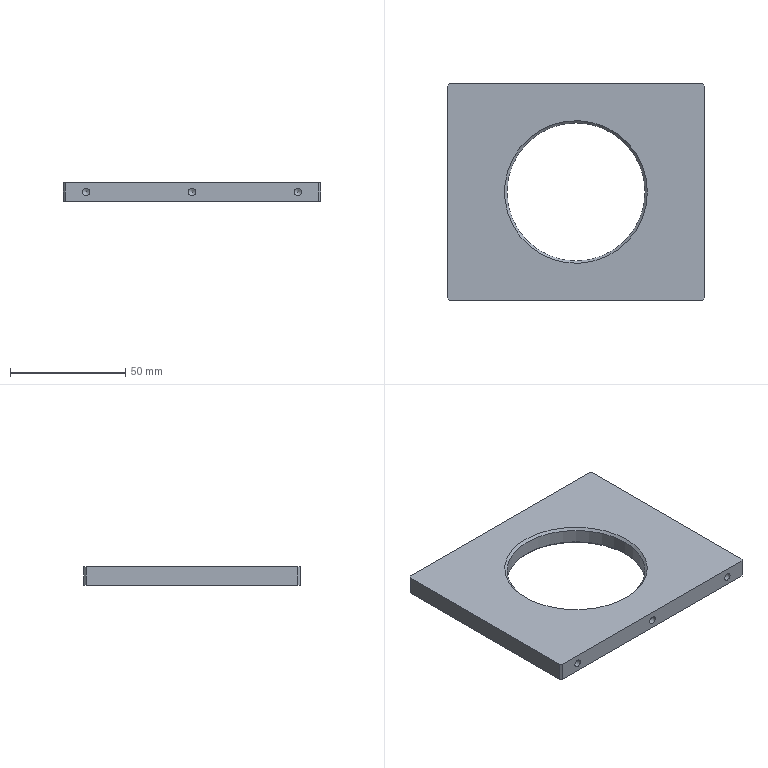Part | NX | 1 solid | 23 faces | box 112 x 94 x 8 mm | volume 60956 mm3 | plane 10 | cone 7 | cylinder 6 | commonest cylinder face diameters 3.3 x5 60 x1
STEP:
#1=CARTESIAN_POINT('',(56.,-34.,-1.65));
#2=VERTEX_POINT('',#1);
#3=CARTESIAN_POINT('',(56.,-34.,0.));
#4=DIRECTION('',(1.,0.,0.));
#5=DIRECTION('',(0.,0.,-1.));
#6=AXIS2_PLACEMENT_3D('',#3,#4,#5);
#7=CIRCLE('',#6,1.65);
#8=EDGE_CURVE('',#2,#2,#7,.T.);
#9=ORIENTED_EDGE('',*,*,#8,.F.);
#10=EDGE_LOOP('',(#9));
#11=FACE_BOUND('',#10,.T.);
#12=CARTESIAN_POINT('',(56.,26.,-1.65));
#13=VERTEX_POINT('',#12);
#14=CARTESIAN_POINT('',(56.,26.,0.));
#15=DIRECTION('',(1.,0.,0.));
#16=DIRECTION('',(0.,0.,-1.));
#17=AXIS2_PLACEMENT_3D('',#14,#15,#16);
#18=CIRCLE('',#17,1.65);
#19=EDGE_CURVE('',#13,#13,#18,.T.);
#20=ORIENTED_EDGE('',*,*,#19,.F.);
#21=EDGE_LOOP('',(#20));
#22=FACE_BOUND('',#21,.T.);
#23=CARTESIAN_POINT('',(56.,-46.,4.));
#24=VERTEX_POINT('',#23);
#25=CARTESIAN_POINT('',(56.,46.,4.));
#26=VERTEX_POINT('',#25);
#27=CARTESIAN_POINT('',(56.,47.,4.));
#28=DIRECTION('',(0.,1.,0.));
#29=VECTOR('',#28,1000.);
#30=LINE('',#27,#29);
#31=EDGE_CURVE('',#24,#26,#30,.T.);
#32=ORIENTED_EDGE('',*,*,#31,.F.);
#33=CARTESIAN_POINT('',(56.,-46.,-4.));
#34=VERTEX_POINT('',#33);
#35=CARTESIAN_POINT('',(56.,-46.,4.));
#36=DIRECTION('',(0.,0.,-1.));
#37=VECTOR('',#36,1000.);
#38=LINE('',#35,#37);
#39=EDGE_CURVE('',#24,#34,#38,.T.);
#40=ORIENTED_EDGE('',*,*,#39,.T.);
#41=CARTESIAN_POINT('',(56.,46.,-4.));
#42=VERTEX_POINT('',#41);
#43=CARTESIAN_POINT('',(56.,47.,-4.));
#44=DIRECTION('',(0.,1.,0.));
#45=VECTOR('',#44,1000.);
#46=LINE('',#43,#45);
#47=EDGE_CURVE('',#34,#42,#46,.T.);
#48=ORIENTED_EDGE('',*,*,#47,.T.);
#49=CARTESIAN_POINT('',(56.,46.,4.));
#50=DIRECTION('',(0.,0.,1.));
#51=VECTOR('',#50,1000.);
#52=LINE('',#49,#51);
#53=EDGE_CURVE('',#42,#26,#52,.T.);
#54=ORIENTED_EDGE('',*,*,#53,.T.);
#55=EDGE_LOOP('',(#32,#40,#48,#54));
#56=FACE_BOUND('',#55,.T.);
#57=CARTESIAN_POINT('',(56.,47.,4.));
#58=DIRECTION('',(-1.,0.,0.));
#59=DIRECTION('',(0.,-1.,0.));
#60=AXIS2_PLACEMENT_3D('',#57,#58,#59);
#61=PLANE('',#60);
#62=ADVANCED_FACE('',(#11,#22,#56),#61,.F.);
#63=CARTESIAN_POINT('',(55.,47.,4.));
#64=VERTEX_POINT('',#63);
#65=CARTESIAN_POINT('',(-55.,47.,4.));
#66=VERTEX_POINT('',#65);
#67=CARTESIAN_POINT('',(-56.,47.,4.));
#68=DIRECTION('',(-1.,0.,0.));
#69=VECTOR('',#68,1000.);
#70=LINE('',#67,#69);
#71=EDGE_CURVE('',#64,#66,#70,.T.);
#72=ORIENTED_EDGE('',*,*,#71,.F.);
#73=CARTESIAN_POINT('',(55.,47.,-4.));
#74=VERTEX_POINT('',#73);
#75=CARTESIAN_POINT('',(55.,47.,4.));
#76=DIRECTION('',(0.,0.,-1.));
#77=VECTOR('',#76,1000.);
#78=LINE('',#75,#77);
#79=EDGE_CURVE('',#64,#74,#78,.T.);
#80=ORIENTED_EDGE('',*,*,#79,.T.);
#81=CARTESIAN_POINT('',(-55.,47.,-4.));
#82=VERTEX_POINT('',#81);
#83=CARTESIAN_POINT('',(-56.,47.,-4.));
#84=DIRECTION('',(-1.,0.,0.));
#85=VECTOR('',#84,1000.);
#86=LINE('',#83,#85);
#87=EDGE_CURVE('',#74,#82,#86,.T.);
#88=ORIENTED_EDGE('',*,*,#87,.T.);
#89=CARTESIAN_POINT('',(-55.,47.,4.));
#90=DIRECTION('',(0.,0.,1.));
#91=VECTOR('',#90,1000.);
#92=LINE('',#89,#91);
#93=EDGE_CURVE('',#82,#66,#92,.T.);
#94=ORIENTED_EDGE('',*,*,#93,.T.);
#95=EDGE_LOOP('',(#72,#80,#88,#94));
#96=FACE_BOUND('',#95,.T.);
#97=CARTESIAN_POINT('',(-56.,47.,4.));
#98=DIRECTION('',(0.,-1.,0.));
#99=DIRECTION('',(0.,0.,-1.));
#100=AXIS2_PLACEMENT_3D('',#97,#98,#99);
#101=PLANE('',#100);
#102=ADVANCED_FACE('',(#96),#101,.F.);
#103=CARTESIAN_POINT('',(-56.,46.,-4.));
#104=VERTEX_POINT('',#103);
#105=CARTESIAN_POINT('',(-56.,-46.,-4.));
#106=VERTEX_POINT('',#105);
#107=CARTESIAN_POINT('',(-56.,47.,-4.));
#108=DIRECTION('',(0.,-1.,0.));
#109=VECTOR('',#108,1000.);
#110=LINE('',#107,#109);
#111=EDGE_CURVE('',#104,#106,#110,.T.);
#112=ORIENTED_EDGE('',*,*,#111,.T.);
#113=CARTESIAN_POINT('',(-56.,-46.,4.));
#114=VERTEX_POINT('',#113);
#115=CARTESIAN_POINT('',(-56.,-46.,4.));
#116=DIRECTION('',(0.,0.,1.));
#117=VECTOR('',#116,1000.);
#118=LINE('',#115,#117);
#119=EDGE_CURVE('',#106,#114,#118,.T.);
#120=ORIENTED_EDGE('',*,*,#119,.T.);
#121=CARTESIAN_POINT('',(-56.,46.,4.));
#122=VERTEX_POINT('',#121);
#123=CARTESIAN_POINT('',(-56.,47.,4.));
#124=DIRECTION('',(0.,-1.,0.));
#125=VECTOR('',#124,1000.);
#126=LINE('',#123,#125);
#127=EDGE_CURVE('',#122,#114,#126,.T.);
#128=ORIENTED_EDGE('',*,*,#127,.F.);
#129=CARTESIAN_POINT('',(-56.,46.,4.));
#130=DIRECTION('',(0.,0.,-1.));
#131=VECTOR('',#130,1000.);
#132=LINE('',#129,#131);
#133=EDGE_CURVE('',#122,#104,#132,.T.);
#134=ORIENTED_EDGE('',*,*,#133,.T.);
#135=EDGE_LOOP('',(#112,#120,#128,#134));
#136=FACE_BOUND('',#135,.T.);
#137=CARTESIAN_POINT('',(-56.,47.,4.));
#138=DIRECTION('',(1.,0.,0.));
#139=DIRECTION('',(0.,1.,0.));
#140=AXIS2_PLACEMENT_3D('',#137,#138,#139);
#141=PLANE('',#140);
#142=ADVANCED_FACE('',(#136),#141,.F.);
#143=CARTESIAN_POINT('',(46.,-47.,-1.65));
#144=VERTEX_POINT('',#143);
#145=CARTESIAN_POINT('',(46.,-47.,0.));
#146=DIRECTION('',(0.,-1.,0.));
#147=DIRECTION('',(0.,0.,-1.));
#148=AXIS2_PLACEMENT_3D('',#145,#146,#147);
#149=CIRCLE('',#148,1.65);
#150=EDGE_CURVE('',#144,#144,#149,.T.);
#151=ORIENTED_EDGE('',*,*,#150,.F.);
#152=EDGE_LOOP('',(#151));
#153=FACE_BOUND('',#152,.T.);
#154=CARTESIAN_POINT('',(0.,-47.,-1.65));
#155=VERTEX_POINT('',#154);
#156=CARTESIAN_POINT('',(0.,-47.,0.));
#157=DIRECTION('',(0.,-1.,0.));
#158=DIRECTION('',(0.,0.,-1.));
#159=AXIS2_PLACEMENT_3D('',#156,#157,#158);
#160=CIRCLE('',#159,1.65);
#161=EDGE_CURVE('',#155,#155,#160,.T.);
#162=ORIENTED_EDGE('',*,*,#161,.F.);
#163=EDGE_LOOP('',(#162));
#164=FACE_BOUND('',#163,.T.);
#165=CARTESIAN_POINT('',(-46.,-47.,-1.65));
#166=VERTEX_POINT('',#165);
#167=CARTESIAN_POINT('',(-46.,-47.,0.));
#168=DIRECTION('',(0.,-1.,0.));
#169=DIRECTION('',(0.,0.,-1.));
#170=AXIS2_PLACEMENT_3D('',#167,#168,#169);
#171=CIRCLE('',#170,1.65);
#172=EDGE_CURVE('',#166,#166,#171,.T.);
#173=ORIENTED_EDGE('',*,*,#172,.F.);
#174=EDGE_LOOP('',(#173));
#175=FACE_BOUND('',#174,.T.);
#176=CARTESIAN_POINT('',(-55.,-47.,-4.));
#177=VERTEX_POINT('',#176);
#178=CARTESIAN_POINT('',(55.,-47.,-4.));
#179=VERTEX_POINT('',#178);
#180=CARTESIAN_POINT('',(-56.,-47.,-4.));
#181=DIRECTION('',(1.,0.,0.));
#182=VECTOR('',#181,1000.);
#183=LINE('',#180,#182);
#184=EDGE_CURVE('',#177,#179,#183,.T.);
#185=ORIENTED_EDGE('',*,*,#184,.T.);
#186=CARTESIAN_POINT('',(55.,-47.,4.));
#187=VERTEX_POINT('',#186);
#188=CARTESIAN_POINT('',(55.,-47.,4.));
#189=DIRECTION('',(0.,0.,1.));
#190=VECTOR('',#189,1000.);
#191=LINE('',#188,#190);
#192=EDGE_CURVE('',#179,#187,#191,.T.);
#193=ORIENTED_EDGE('',*,*,#192,.T.);
#194=CARTESIAN_POINT('',(-55.,-47.,4.));
#195=VERTEX_POINT('',#194);
#196=CARTESIAN_POINT('',(-56.,-47.,4.));
#197=DIRECTION('',(1.,0.,0.));
#198=VECTOR('',#197,1000.);
#199=LINE('',#196,#198);
#200=EDGE_CURVE('',#195,#187,#199,.T.);
#201=ORIENTED_EDGE('',*,*,#200,.F.);
#202=CARTESIAN_POINT('',(-55.,-47.,4.));
#203=DIRECTION('',(0.,0.,-1.));
#204=VECTOR('',#203,1000.);
#205=LINE('',#202,#204);
#206=EDGE_CURVE('',#195,#177,#205,.T.);
#207=ORIENTED_EDGE('',*,*,#206,.T.);
#208=EDGE_LOOP('',(#185,#193,#201,#207));
#209=FACE_BOUND('',#208,.T.);
#210=CARTESIAN_POINT('',(-56.,-47.,4.));
#211=DIRECTION('',(0.,1.,0.));
#212=DIRECTION('',(0.,0.,1.));
#213=AXIS2_PLACEMENT_3D('',#210,#211,#212);
#214=PLANE('',#213);
#215=ADVANCED_FACE('',(#153,#164,#175,#209),#214,.F.);
#216=CARTESIAN_POINT('',(31.,0.,4.));
#217=VERTEX_POINT('',#216);
#218=CARTESIAN_POINT('',(0.,0.,4.));
#219=DIRECTION('',(0.,0.,1.));
#220=DIRECTION('',(1.,0.,0.));
#221=AXIS2_PLACEMENT_3D('',#218,#219,#220);
#222=CIRCLE('',#221,31.);
#223=EDGE_CURVE('',#217,#217,#222,.F.);
#224=ORIENTED_EDGE('',*,*,#223,.T.);
#225=EDGE_LOOP('',(#224));
#226=FACE_BOUND('',#225,.T.);
#227=ORIENTED_EDGE('',*,*,#200,.T.);
#228=CARTESIAN_POINT('',(51.,-51.,4.));
#229=DIRECTION('',(-0.7071,-0.7071,0.));
#230=VECTOR('',#229,1000.);
#231=LINE('',#228,#230);
#232=EDGE_CURVE('',#187,#24,#231,.F.);
#233=ORIENTED_EDGE('',*,*,#232,.T.);
#234=ORIENTED_EDGE('',*,*,#31,.T.);
#235=CARTESIAN_POINT('',(51.,51.,4.));
#236=DIRECTION('',(0.7071,-0.7071,0.));
#237=VECTOR('',#236,1000.);
#238=LINE('',#235,#237);
#239=EDGE_CURVE('',#26,#64,#238,.F.);
#240=ORIENTED_EDGE('',*,*,#239,.T.);
#241=ORIENTED_EDGE('',*,*,#71,.T.);
#242=CARTESIAN_POINT('',(-51.,51.,4.));
#243=DIRECTION('',(0.7071,0.7071,0.));
#244=VECTOR('',#243,1000.);
#245=LINE('',#242,#244);
#246=EDGE_CURVE('',#66,#122,#245,.F.);
#247=ORIENTED_EDGE('',*,*,#246,.T.);
#248=ORIENTED_EDGE('',*,*,#127,.T.);
#249=CARTESIAN_POINT('',(-51.,-51.,4.));
#250=DIRECTION('',(-0.7071,0.7071,0.));
#251=VECTOR('',#250,1000.);
#252=LINE('',#249,#251);
#253=EDGE_CURVE('',#114,#195,#252,.F.);
#254=ORIENTED_EDGE('',*,*,#253,.T.);
#255=EDGE_LOOP('',(#227,#233,#234,#240,#241,#247,#248,#254));
#256=FACE_BOUND('',#255,.T.);
#257=CARTESIAN_POINT('',(0.,0.,4.));
#258=DIRECTION('',(0.,0.,1.));
#259=DIRECTION('',(1.,0.,0.));
#260=AXIS2_PLACEMENT_3D('',#257,#258,#259);
#261=PLANE('',#260);
#262=ADVANCED_FACE('',(#226,#256),#261,.T.);
#263=CARTESIAN_POINT('',(31.,0.,-4.));
#264=VERTEX_POINT('',#263);
#265=CARTESIAN_POINT('',(0.,0.,-4.));
#266=DIRECTION('',(0.,0.,1.));
#267=DIRECTION('',(1.,0.,0.));
#268=AXIS2_PLACEMENT_3D('',#265,#266,#267);
#269=CIRCLE('',#268,31.);
#270=EDGE_CURVE('',#264,#264,#269,.T.);
#271=ORIENTED_EDGE('',*,*,#270,.T.);
#272=EDGE_LOOP('',(#271));
#273=FACE_BOUND('',#272,.T.);
#274=ORIENTED_EDGE('',*,*,#47,.F.);
#275=CARTESIAN_POINT('',(56.,-46.,-4.));
#276=DIRECTION('',(0.7071,0.7071,0.));
#277=VECTOR('',#276,1000.);
#278=LINE('',#275,#277);
#279=EDGE_CURVE('',#34,#179,#278,.F.);
#280=ORIENTED_EDGE('',*,*,#279,.T.);
#281=ORIENTED_EDGE('',*,*,#184,.F.);
#282=CARTESIAN_POINT('',(-55.,-47.,-4.));
#283=DIRECTION('',(0.7071,-0.7071,0.));
#284=VECTOR('',#283,1000.);
#285=LINE('',#282,#284);
#286=EDGE_CURVE('',#177,#106,#285,.F.);
#287=ORIENTED_EDGE('',*,*,#286,.T.);
#288=ORIENTED_EDGE('',*,*,#111,.F.);
#289=CARTESIAN_POINT('',(-56.,46.,-4.));
#290=DIRECTION('',(-0.7071,-0.7071,0.));
#291=VECTOR('',#290,1000.);
#292=LINE('',#289,#291);
#293=EDGE_CURVE('',#104,#82,#292,.F.);
#294=ORIENTED_EDGE('',*,*,#293,.T.);
#295=ORIENTED_EDGE('',*,*,#87,.F.);
#296=CARTESIAN_POINT('',(55.,47.,-4.));
#297=DIRECTION('',(-0.7071,0.7071,0.));
#298=VECTOR('',#297,1000.);
#299=LINE('',#296,#298);
#300=EDGE_CURVE('',#74,#42,#299,.F.);
#301=ORIENTED_EDGE('',*,*,#300,.T.);
#302=EDGE_LOOP('',(#274,#280,#281,#287,#288,#294,#295,#301));
#303=FACE_BOUND('',#302,.T.);
#304=CARTESIAN_POINT('',(0.,0.,-4.));
#305=DIRECTION('',(0.,0.,1.));
#306=DIRECTION('',(1.,0.,0.));
#307=AXIS2_PLACEMENT_3D('',#304,#305,#306);
#308=PLANE('',#307);
#309=ADVANCED_FACE('',(#273,#303),#308,.F.);
#310=CARTESIAN_POINT('',(30.,0.,-3.));
#311=VERTEX_POINT('',#310);
#312=CARTESIAN_POINT('',(0.,0.,-3.));
#313=DIRECTION('',(0.,0.,1.));
#314=DIRECTION('',(1.,0.,0.));
#315=AXIS2_PLACEMENT_3D('',#312,#313,#314);
#316=CIRCLE('',#315,30.);
#317=EDGE_CURVE('',#311,#311,#316,.F.);
#318=ORIENTED_EDGE('',*,*,#317,.T.);
#319=EDGE_LOOP('',(#318));
#320=FACE_BOUND('',#319,.T.);
#321=CARTESIAN_POINT('',(30.,0.,3.));
#322=VERTEX_POINT('',#321);
#323=CARTESIAN_POINT('',(0.,0.,3.));
#324=DIRECTION('',(0.,0.,1.));
#325=DIRECTION('',(1.,0.,0.));
#326=AXIS2_PLACEMENT_3D('',#323,#324,#325);
#327=CIRCLE('',#326,30.);
#328=EDGE_CURVE('',#322,#322,#327,.T.);
#329=ORIENTED_EDGE('',*,*,#328,.T.);
#330=EDGE_LOOP('',(#329));
#331=FACE_BOUND('',#330,.T.);
#332=CARTESIAN_POINT('',(0.,0.,4.));
#333=DIRECTION('',(0.,0.,-1.));
#334=DIRECTION('',(-1.,0.,0.));
#335=AXIS2_PLACEMENT_3D('',#332,#333,#334);
#336=CYLINDRICAL_SURFACE('',#335,30.);
#337=ADVANCED_FACE('',(#320,#331),#336,.F.);
#338=CARTESIAN_POINT('',(45.009,26.,0.));
#339=VERTEX_POINT('',#338);
#340=VERTEX_LOOP('',#339);
#341=FACE_BOUND('',#340,.T.);
#342=CARTESIAN_POINT('',(46.,26.,-1.65));
#343=VERTEX_POINT('',#342);
#344=CARTESIAN_POINT('',(46.,26.,0.));
#345=DIRECTION('',(1.,0.,0.));
#346=DIRECTION('',(0.,0.,-1.));
#347=AXIS2_PLACEMENT_3D('',#344,#345,#346);
#348=CIRCLE('',#347,1.65);
#349=EDGE_CURVE('',#343,#343,#348,.T.);
#350=ORIENTED_EDGE('',*,*,#349,.T.);
#351=EDGE_LOOP('',(#350));
#352=FACE_BOUND('',#351,.T.);
#353=CARTESIAN_POINT('',(46.,26.,0.));
#354=DIRECTION('',(1.,0.,0.));
#355=DIRECTION('',(0.,0.,-1.));
#356=AXIS2_PLACEMENT_3D('',#353,#354,#355);
#357=CONICAL_SURFACE('',#356,1.65,1.03);
#358=ADVANCED_FACE('',(#341,#352),#357,.F.);
#359=ORIENTED_EDGE('',*,*,#349,.F.);
#360=EDGE_LOOP('',(#359));
#361=FACE_BOUND('',#360,.T.);
#362=ORIENTED_EDGE('',*,*,#19,.T.);
#363=EDGE_LOOP('',(#362));
#364=FACE_BOUND('',#363,.T.);
#365=CARTESIAN_POINT('',(56.,26.,0.));
#366=DIRECTION('',(1.,0.,0.));
#367=DIRECTION('',(0.,0.,-1.));
#368=AXIS2_PLACEMENT_3D('',#365,#366,#367);
#369=CYLINDRICAL_SURFACE('',#368,1.65);
#370=ADVANCED_FACE('',(#361,#364),#369,.F.);
#371=CARTESIAN_POINT('',(45.009,-34.,0.));
#372=VERTEX_POINT('',#371);
#373=VERTEX_LOOP('',#372);
#374=FACE_BOUND('',#373,.T.);
#375=CARTESIAN_POINT('',(46.,-34.,-1.65));
#376=VERTEX_POINT('',#375);
#377=CARTESIAN_POINT('',(46.,-34.,0.));
#378=DIRECTION('',(1.,0.,0.));
#379=DIRECTION('',(0.,0.,-1.));
#380=AXIS2_PLACEMENT_3D('',#377,#378,#379);
#381=CIRCLE('',#380,1.65);
#382=EDGE_CURVE('',#376,#376,#381,.T.);
#383=ORIENTED_EDGE('',*,*,#382,.T.);
#384=EDGE_LOOP('',(#383));
#385=FACE_BOUND('',#384,.T.);
#386=CARTESIAN_POINT('',(46.,-34.,0.));
#387=DIRECTION('',(1.,0.,0.));
#388=DIRECTION('',(0.,0.,-1.));
#389=AXIS2_PLACEMENT_3D('',#386,#387,#388);
#390=CONICAL_SURFACE('',#389,1.65,1.03);
#391=ADVANCED_FACE('',(#374,#385),#390,.F.);
#392=ORIENTED_EDGE('',*,*,#382,.F.);
#393=EDGE_LOOP('',(#392));
#394=FACE_BOUND('',#393,.T.);
#395=ORIENTED_EDGE('',*,*,#8,.T.);
#396=EDGE_LOOP('',(#395));
#397=FACE_BOUND('',#396,.T.);
#398=CARTESIAN_POINT('',(56.,-34.,0.));
#399=DIRECTION('',(1.,0.,0.));
#400=DIRECTION('',(0.,0.,-1.));
#401=AXIS2_PLACEMENT_3D('',#398,#399,#400);
#402=CYLINDRICAL_SURFACE('',#401,1.65);
#403=ADVANCED_FACE('',(#394,#397),#402,.F.);
#404=CARTESIAN_POINT('',(-46.,-36.009,0.));
#405=VERTEX_POINT('',#404);
#406=VERTEX_LOOP('',#405);
#407=FACE_BOUND('',#406,.T.);
#408=CARTESIAN_POINT('',(-46.,-37.,-1.65));
#409=VERTEX_POINT('',#408);
#410=CARTESIAN_POINT('',(-46.,-37.,0.));
#411=DIRECTION('',(0.,-1.,0.));
#412=DIRECTION('',(0.,0.,-1.));
#413=AXIS2_PLACEMENT_3D('',#410,#411,#412);
#414=CIRCLE('',#413,1.65);
#415=EDGE_CURVE('',#409,#409,#414,.T.);
#416=ORIENTED_EDGE('',*,*,#415,.T.);
#417=EDGE_LOOP('',(#416));
#418=FACE_BOUND('',#417,.T.);
#419=CARTESIAN_POINT('',(-46.,-37.,0.));
#420=DIRECTION('',(0.,-1.,0.));
#421=DIRECTION('',(0.,0.,-1.));
#422=AXIS2_PLACEMENT_3D('',#419,#420,#421);
#423=CONICAL_SURFACE('',#422,1.65,1.03);
#424=ADVANCED_FACE('',(#407,#418),#423,.F.);
#425=ORIENTED_EDGE('',*,*,#415,.F.);
#426=EDGE_LOOP('',(#425));
#427=FACE_BOUND('',#426,.T.);
#428=ORIENTED_EDGE('',*,*,#172,.T.);
#429=EDGE_LOOP('',(#428));
#430=FACE_BOUND('',#429,.T.);
#431=CARTESIAN_POINT('',(-46.,-47.,0.));
#432=DIRECTION('',(0.,-1.,0.));
#433=DIRECTION('',(0.,0.,-1.));
#434=AXIS2_PLACEMENT_3D('',#431,#432,#433);
#435=CYLINDRICAL_SURFACE('',#434,1.65);
#436=ADVANCED_FACE('',(#427,#430),#435,.F.);
#437=CARTESIAN_POINT('',(0.,-36.009,0.));
#438=VERTEX_POINT('',#437);
#439=VERTEX_LOOP('',#438);
#440=FACE_BOUND('',#439,.T.);
#441=CARTESIAN_POINT('',(0.,-37.,-1.65));
#442=VERTEX_POINT('',#441);
#443=CARTESIAN_POINT('',(0.,-37.,0.));
#444=DIRECTION('',(0.,-1.,0.));
#445=DIRECTION('',(0.,0.,-1.));
#446=AXIS2_PLACEMENT_3D('',#443,#444,#445);
#447=CIRCLE('',#446,1.65);
#448=EDGE_CURVE('',#442,#442,#447,.T.);
#449=ORIENTED_EDGE('',*,*,#448,.T.);
#450=EDGE_LOOP('',(#449));
#451=FACE_BOUND('',#450,.T.);
#452=CARTESIAN_POINT('',(0.,-37.,0.));
#453=DIRECTION('',(0.,-1.,0.));
#454=DIRECTION('',(0.,0.,-1.));
#455=AXIS2_PLACEMENT_3D('',#452,#453,#454);
#456=CONICAL_SURFACE('',#455,1.65,1.03);
#457=ADVANCED_FACE('',(#440,#451),#456,.F.);
#458=ORIENTED_EDGE('',*,*,#448,.F.);
#459=EDGE_LOOP('',(#458));
#460=FACE_BOUND('',#459,.T.);
#461=ORIENTED_EDGE('',*,*,#161,.T.);
#462=EDGE_LOOP('',(#461));
#463=FACE_BOUND('',#462,.T.);
#464=CARTESIAN_POINT('',(0.,-47.,0.));
#465=DIRECTION('',(0.,-1.,0.));
#466=DIRECTION('',(0.,0.,-1.));
#467=AXIS2_PLACEMENT_3D('',#464,#465,#466);
#468=CYLINDRICAL_SURFACE('',#467,1.65);
#469=ADVANCED_FACE('',(#460,#463),#468,.F.);
#470=CARTESIAN_POINT('',(46.,-36.009,0.));
#471=VERTEX_POINT('',#470);
#472=VERTEX_LOOP('',#471);
#473=FACE_BOUND('',#472,.T.);
#474=CARTESIAN_POINT('',(46.,-37.,-1.65));
#475=VERTEX_POINT('',#474);
#476=CARTESIAN_POINT('',(46.,-37.,0.));
#477=DIRECTION('',(0.,-1.,0.));
#478=DIRECTION('',(0.,0.,-1.));
#479=AXIS2_PLACEMENT_3D('',#476,#477,#478);
#480=CIRCLE('',#479,1.65);
#481=EDGE_CURVE('',#475,#475,#480,.T.);
#482=ORIENTED_EDGE('',*,*,#481,.T.);
#483=EDGE_LOOP('',(#482));
#484=FACE_BOUND('',#483,.T.);
#485=CARTESIAN_POINT('',(46.,-37.,0.));
#486=DIRECTION('',(0.,-1.,0.));
#487=DIRECTION('',(0.,0.,-1.));
#488=AXIS2_PLACEMENT_3D('',#485,#486,#487);
#489=CONICAL_SURFACE('',#488,1.65,1.03);
#490=ADVANCED_FACE('',(#473,#484),#489,.F.);
#491=ORIENTED_EDGE('',*,*,#481,.F.);
#492=EDGE_LOOP('',(#491));
#493=FACE_BOUND('',#492,.T.);
#494=ORIENTED_EDGE('',*,*,#150,.T.);
#495=EDGE_LOOP('',(#494));
#496=FACE_BOUND('',#495,.T.);
#497=CARTESIAN_POINT('',(46.,-47.,0.));
#498=DIRECTION('',(0.,-1.,0.));
#499=DIRECTION('',(0.,0.,-1.));
#500=AXIS2_PLACEMENT_3D('',#497,#498,#499);
#501=CYLINDRICAL_SURFACE('',#500,1.65);
#502=ADVANCED_FACE('',(#493,#496),#501,.F.);
#503=ORIENTED_EDGE('',*,*,#232,.F.);
#504=ORIENTED_EDGE('',*,*,#192,.F.);
#505=ORIENTED_EDGE('',*,*,#279,.F.);
#506=ORIENTED_EDGE('',*,*,#39,.F.);
#507=EDGE_LOOP('',(#503,#504,#505,#506));
#508=FACE_BOUND('',#507,.T.);
#509=CARTESIAN_POINT('',(56.,-46.,4.));
#510=DIRECTION('',(-0.7071,0.7071,0.));
#511=DIRECTION('',(0.,0.,-1.));
#512=AXIS2_PLACEMENT_3D('',#509,#510,#511);
#513=PLANE('',#512);
#514=ADVANCED_FACE('',(#508),#513,.F.);
#515=ORIENTED_EDGE('',*,*,#253,.F.);
#516=ORIENTED_EDGE('',*,*,#119,.F.);
#517=ORIENTED_EDGE('',*,*,#286,.F.);
#518=ORIENTED_EDGE('',*,*,#206,.F.);
#519=EDGE_LOOP('',(#515,#516,#517,#518));
#520=FACE_BOUND('',#519,.T.);
#521=CARTESIAN_POINT('',(-55.,-47.,4.));
#522=DIRECTION('',(0.7071,0.7071,0.));
#523=DIRECTION('',(0.,0.,-1.));
#524=AXIS2_PLACEMENT_3D('',#521,#522,#523);
#525=PLANE('',#524);
#526=ADVANCED_FACE('',(#520),#525,.F.);
#527=ORIENTED_EDGE('',*,*,#239,.F.);
#528=ORIENTED_EDGE('',*,*,#53,.F.);
#529=ORIENTED_EDGE('',*,*,#300,.F.);
#530=ORIENTED_EDGE('',*,*,#79,.F.);
#531=EDGE_LOOP('',(#527,#528,#529,#530));
#532=FACE_BOUND('',#531,.T.);
#533=CARTESIAN_POINT('',(55.,47.,4.));
#534=DIRECTION('',(-0.7071,-0.7071,0.));
#535=DIRECTION('',(0.,0.,-1.));
#536=AXIS2_PLACEMENT_3D('',#533,#534,#535);
#537=PLANE('',#536);
#538=ADVANCED_FACE('',(#532),#537,.F.);
#539=ORIENTED_EDGE('',*,*,#246,.F.);
#540=ORIENTED_EDGE('',*,*,#93,.F.);
#541=ORIENTED_EDGE('',*,*,#293,.F.);
#542=ORIENTED_EDGE('',*,*,#133,.F.);
#543=EDGE_LOOP('',(#539,#540,#541,#542));
#544=FACE_BOUND('',#543,.T.);
#545=CARTESIAN_POINT('',(-56.,46.,4.));
#546=DIRECTION('',(0.7071,-0.7071,0.));
#547=DIRECTION('',(0.,0.,-1.));
#548=AXIS2_PLACEMENT_3D('',#545,#546,#547);
#549=PLANE('',#548);
#550=ADVANCED_FACE('',(#544),#549,.F.);
#551=ORIENTED_EDGE('',*,*,#270,.F.);
#552=EDGE_LOOP('',(#551));
#553=FACE_BOUND('',#552,.T.);
#554=ORIENTED_EDGE('',*,*,#317,.F.);
#555=EDGE_LOOP('',(#554));
#556=FACE_BOUND('',#555,.T.);
#557=CARTESIAN_POINT('',(0.,0.,-3.));
#558=DIRECTION('',(0.,0.,-1.));
#559=DIRECTION('',(-1.,0.,0.));
#560=AXIS2_PLACEMENT_3D('',#557,#558,#559);
#561=CONICAL_SURFACE('',#560,30.,0.7854);
#562=ADVANCED_FACE('',(#553,#556),#561,.F.);
#563=ORIENTED_EDGE('',*,*,#328,.F.);
#564=EDGE_LOOP('',(#563));
#565=FACE_BOUND('',#564,.T.);
#566=ORIENTED_EDGE('',*,*,#223,.F.);
#567=EDGE_LOOP('',(#566));
#568=FACE_BOUND('',#567,.T.);
#569=CARTESIAN_POINT('',(0.,0.,4.));
#570=DIRECTION('',(0.,0.,1.));
#571=DIRECTION('',(1.,0.,0.));
#572=AXIS2_PLACEMENT_3D('',#569,#570,#571);
#573=CONICAL_SURFACE('',#572,31.,0.7854);
#574=ADVANCED_FACE('',(#565,#568),#573,.F.);
#575=CLOSED_SHELL('',(#62,#102,#142,#215,#262,#309,#337,#358,#370,#391,#403,#424,#436,#457,#469,#490,#502,#514,#526,#538,#550,#562,#574));
#576=MANIFOLD_SOLID_BREP('',#575);
#577=(LENGTH_UNIT()NAMED_UNIT(*)SI_UNIT(.MILLI.,.METRE.));
#578=UNCERTAINTY_MEASURE_WITH_UNIT(LENGTH_MEASURE(0.00001),#577,'','');
#579=(NAMED_UNIT(*)PLANE_ANGLE_UNIT()SI_UNIT($,.RADIAN.));
#580=(NAMED_UNIT(*)SI_UNIT($,.STERADIAN.)SOLID_ANGLE_UNIT());
#581=(GEOMETRIC_REPRESENTATION_CONTEXT(3)GLOBAL_UNCERTAINTY_ASSIGNED_CONTEXT((#578))GLOBAL_UNIT_ASSIGNED_CONTEXT((#577,#579,#580))REPRESENTATION_CONTEXT('',''));
#582=ADVANCED_BREP_SHAPE_REPRESENTATION('',(#576),#581);